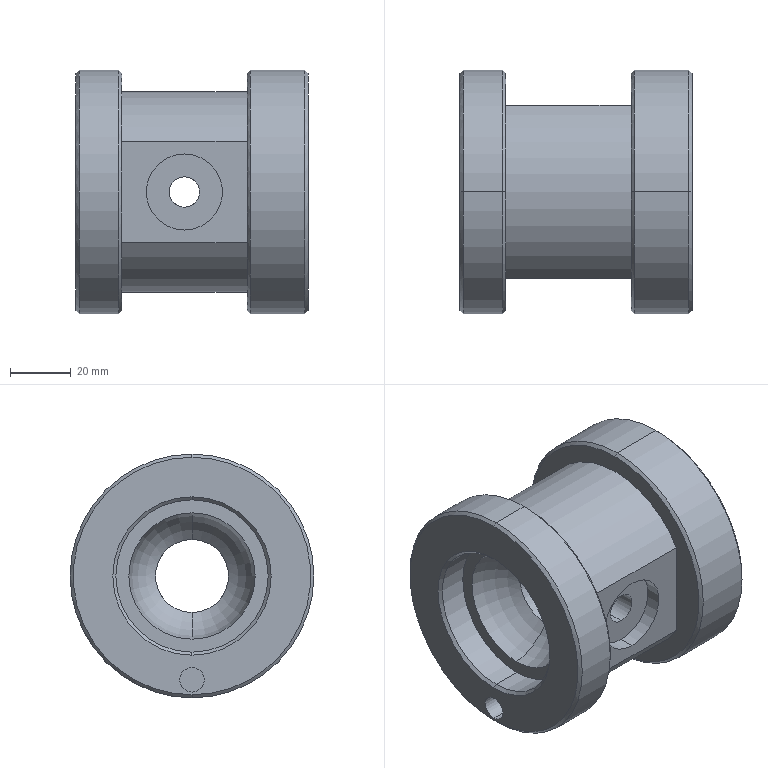Part | SolidWorks | features ICE 5, Chamfer 1, MirrorPattern 1, Revolution 1 | 1 solid | 63 faces | box 76.2 x 80 x 80 mm | volume 211885 mm3 | cylinder 28 | cone 19 | plane 14 | torus 2 | commonest cylinder face diameters 8 x4 10 x4 25 x4 80 x4 29.3 x3 66 x3